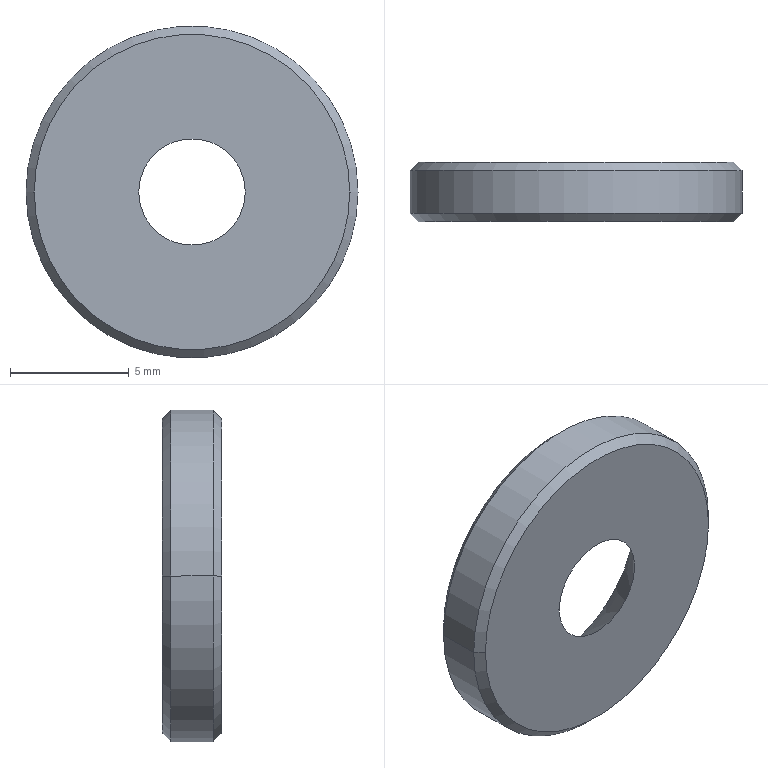Part | NX | 1 solid | 10 faces | box 14 x 2.5 x 14 mm | volume 279.245 mm3 | cone 6 | cylinder 2 | plane 2 | commonest cylinder face diameters 14 x2
STEP:
#1=CARTESIAN_POINT('',(-4.75,2.5,0.));
#2=VERTEX_POINT('',#1);
#3=CARTESIAN_POINT('',(4.75,2.5,0.));
#4=VERTEX_POINT('',#3);
#5=CARTESIAN_POINT('',(0.,2.5,0.));
#6=DIRECTION('',(0.,1.,0.));
#7=DIRECTION('',(1.,0.,0.));
#8=AXIS2_PLACEMENT_3D('',#5,#6,#7);
#9=CIRCLE('',#8,4.75);
#10=EDGE_CURVE('',#2,#4,#9,.T.);
#11=ORIENTED_EDGE('',*,*,#10,.T.);
#12=CARTESIAN_POINT('',(2.25,0.,0.));
#13=VERTEX_POINT('',#12);
#14=CARTESIAN_POINT('',(3.5,1.25,0.));
#15=DIRECTION('',(0.7071,0.7071,0.));
#16=VECTOR('',#15,1000.);
#17=LINE('',#14,#16);
#18=EDGE_CURVE('',#13,#4,#17,.T.);
#19=ORIENTED_EDGE('',*,*,#18,.F.);
#20=CARTESIAN_POINT('',(-2.25,0.,0.));
#21=VERTEX_POINT('',#20);
#22=CARTESIAN_POINT('',(0.,0.,0.));
#23=DIRECTION('',(0.,1.,0.));
#24=DIRECTION('',(1.,0.,0.));
#25=AXIS2_PLACEMENT_3D('',#22,#23,#24);
#26=CIRCLE('',#25,2.25);
#27=EDGE_CURVE('',#21,#13,#26,.T.);
#28=ORIENTED_EDGE('',*,*,#27,.F.);
#29=CARTESIAN_POINT('',(-3.5,1.25,0.));
#30=DIRECTION('',(-0.7071,0.7071,0.));
#31=VECTOR('',#30,1000.);
#32=LINE('',#29,#31);
#33=EDGE_CURVE('',#21,#2,#32,.T.);
#34=ORIENTED_EDGE('',*,*,#33,.T.);
#35=EDGE_LOOP('',(#11,#19,#28,#34));
#36=FACE_BOUND('',#35,.T.);
#37=CARTESIAN_POINT('',(0.,1.25,0.));
#38=DIRECTION('',(0.,1.,0.));
#39=DIRECTION('',(1.,0.,0.));
#40=AXIS2_PLACEMENT_3D('',#37,#38,#39);
#41=CONICAL_SURFACE('',#40,3.5,0.7854);
#42=ADVANCED_FACE('',(#36),#41,.F.);
#43=CARTESIAN_POINT('',(7.,2.15,0.));
#44=VERTEX_POINT('',#43);
#45=CARTESIAN_POINT('',(-7.,2.15,0.));
#46=VERTEX_POINT('',#45);
#47=CARTESIAN_POINT('',(0.,2.15,0.));
#48=DIRECTION('',(0.,1.,0.));
#49=DIRECTION('',(1.,0.,0.));
#50=AXIS2_PLACEMENT_3D('',#47,#48,#49);
#51=CIRCLE('',#50,7.);
#52=EDGE_CURVE('',#44,#46,#51,.T.);
#53=ORIENTED_EDGE('',*,*,#52,.T.);
#54=CARTESIAN_POINT('',(-6.65,2.5,0.));
#55=VERTEX_POINT('',#54);
#56=CARTESIAN_POINT('',(-6.825,2.325,0.));
#57=DIRECTION('',(-0.7071,-0.7071,0.));
#58=VECTOR('',#57,1000.);
#59=LINE('',#56,#58);
#60=EDGE_CURVE('',#46,#55,#59,.F.);
#61=ORIENTED_EDGE('',*,*,#60,.T.);
#62=CARTESIAN_POINT('',(6.65,2.5,0.));
#63=VERTEX_POINT('',#62);
#64=CARTESIAN_POINT('',(0.,2.5,0.));
#65=DIRECTION('',(0.,1.,0.));
#66=DIRECTION('',(1.,0.,0.));
#67=AXIS2_PLACEMENT_3D('',#64,#65,#66);
#68=CIRCLE('',#67,6.65);
#69=EDGE_CURVE('',#63,#55,#68,.T.);
#70=ORIENTED_EDGE('',*,*,#69,.F.);
#71=CARTESIAN_POINT('',(6.825,2.325,0.));
#72=DIRECTION('',(0.7071,-0.7071,0.));
#73=VECTOR('',#72,1000.);
#74=LINE('',#71,#73);
#75=EDGE_CURVE('',#44,#63,#74,.F.);
#76=ORIENTED_EDGE('',*,*,#75,.F.);
#77=EDGE_LOOP('',(#53,#61,#70,#76));
#78=FACE_BOUND('',#77,.T.);
#79=CARTESIAN_POINT('',(0.,2.325,0.));
#80=DIRECTION('',(0.,-1.,0.));
#81=DIRECTION('',(-1.,0.,0.));
#82=AXIS2_PLACEMENT_3D('',#79,#80,#81);
#83=CONICAL_SURFACE('',#82,6.825,0.7854);
#84=ADVANCED_FACE('',(#78),#83,.T.);
#85=CARTESIAN_POINT('',(7.,0.35,0.));
#86=VERTEX_POINT('',#85);
#87=CARTESIAN_POINT('',(-7.,0.35,0.));
#88=VERTEX_POINT('',#87);
#89=CARTESIAN_POINT('',(0.,0.35,0.));
#90=DIRECTION('',(0.,1.,0.));
#91=DIRECTION('',(1.,0.,0.));
#92=AXIS2_PLACEMENT_3D('',#89,#90,#91);
#93=CIRCLE('',#92,7.);
#94=EDGE_CURVE('',#86,#88,#93,.T.);
#95=ORIENTED_EDGE('',*,*,#94,.T.);
#96=CARTESIAN_POINT('',(-7.,1.25,0.));
#97=DIRECTION('',(0.,-1.,0.));
#98=VECTOR('',#97,1000.);
#99=LINE('',#96,#98);
#100=EDGE_CURVE('',#46,#88,#99,.T.);
#101=ORIENTED_EDGE('',*,*,#100,.F.);
#102=ORIENTED_EDGE('',*,*,#52,.F.);
#103=CARTESIAN_POINT('',(7.,1.25,0.));
#104=DIRECTION('',(0.,-1.,0.));
#105=VECTOR('',#104,1000.);
#106=LINE('',#103,#105);
#107=EDGE_CURVE('',#44,#86,#106,.T.);
#108=ORIENTED_EDGE('',*,*,#107,.T.);
#109=EDGE_LOOP('',(#95,#101,#102,#108));
#110=FACE_BOUND('',#109,.T.);
#111=CARTESIAN_POINT('',(0.,1.25,0.));
#112=DIRECTION('',(0.,-1.,0.));
#113=DIRECTION('',(1.,0.,0.));
#114=AXIS2_PLACEMENT_3D('',#111,#112,#113);
#115=CYLINDRICAL_SURFACE('',#114,7.);
#116=ADVANCED_FACE('',(#110),#115,.T.);
#117=ORIENTED_EDGE('',*,*,#94,.F.);
#118=CARTESIAN_POINT('',(6.65,0.,0.));
#119=VERTEX_POINT('',#118);
#120=CARTESIAN_POINT('',(6.825,0.175,0.));
#121=DIRECTION('',(0.7071,0.7071,0.));
#122=VECTOR('',#121,1000.);
#123=LINE('',#120,#122);
#124=EDGE_CURVE('',#119,#86,#123,.T.);
#125=ORIENTED_EDGE('',*,*,#124,.F.);
#126=CARTESIAN_POINT('',(-6.65,0.,0.));
#127=VERTEX_POINT('',#126);
#128=CARTESIAN_POINT('',(0.,0.,0.));
#129=DIRECTION('',(0.,1.,0.));
#130=DIRECTION('',(1.,0.,0.));
#131=AXIS2_PLACEMENT_3D('',#128,#129,#130);
#132=CIRCLE('',#131,6.65);
#133=EDGE_CURVE('',#119,#127,#132,.T.);
#134=ORIENTED_EDGE('',*,*,#133,.T.);
#135=CARTESIAN_POINT('',(-6.825,0.175,0.));
#136=DIRECTION('',(-0.7071,0.7071,0.));
#137=VECTOR('',#136,1000.);
#138=LINE('',#135,#137);
#139=EDGE_CURVE('',#127,#88,#138,.T.);
#140=ORIENTED_EDGE('',*,*,#139,.T.);
#141=EDGE_LOOP('',(#117,#125,#134,#140));
#142=FACE_BOUND('',#141,.T.);
#143=CARTESIAN_POINT('',(0.,0.175,0.));
#144=DIRECTION('',(0.,1.,0.));
#145=DIRECTION('',(1.,0.,0.));
#146=AXIS2_PLACEMENT_3D('',#143,#144,#145);
#147=CONICAL_SURFACE('',#146,6.825,0.7854);
#148=ADVANCED_FACE('',(#142),#147,.T.);
#149=CARTESIAN_POINT('',(0.,2.5,0.));
#150=DIRECTION('',(0.,1.,0.));
#151=DIRECTION('',(1.,0.,0.));
#152=AXIS2_PLACEMENT_3D('',#149,#150,#151);
#153=CIRCLE('',#152,6.65);
#154=EDGE_CURVE('',#55,#63,#153,.T.);
#155=ORIENTED_EDGE('',*,*,#154,.T.);
#156=ORIENTED_EDGE('',*,*,#69,.T.);
#157=EDGE_LOOP('',(#155,#156));
#158=FACE_BOUND('',#157,.T.);
#159=ORIENTED_EDGE('',*,*,#10,.F.);
#160=CARTESIAN_POINT('',(0.,2.5,0.));
#161=DIRECTION('',(0.,1.,0.));
#162=DIRECTION('',(1.,0.,0.));
#163=AXIS2_PLACEMENT_3D('',#160,#161,#162);
#164=CIRCLE('',#163,4.75);
#165=EDGE_CURVE('',#4,#2,#164,.T.);
#166=ORIENTED_EDGE('',*,*,#165,.F.);
#167=EDGE_LOOP('',(#159,#166));
#168=FACE_BOUND('',#167,.T.);
#169=CARTESIAN_POINT('',(5.7,2.5,0.));
#170=DIRECTION('',(0.,1.,0.));
#171=DIRECTION('',(1.,0.,0.));
#172=AXIS2_PLACEMENT_3D('',#169,#170,#171);
#173=PLANE('',#172);
#174=ADVANCED_FACE('',(#158,#168),#173,.T.);
#175=CARTESIAN_POINT('',(0.,0.,0.));
#176=DIRECTION('',(0.,1.,0.));
#177=DIRECTION('',(1.,0.,0.));
#178=AXIS2_PLACEMENT_3D('',#175,#176,#177);
#179=CIRCLE('',#178,6.65);
#180=EDGE_CURVE('',#127,#119,#179,.T.);
#181=ORIENTED_EDGE('',*,*,#180,.F.);
#182=ORIENTED_EDGE('',*,*,#133,.F.);
#183=EDGE_LOOP('',(#181,#182));
#184=FACE_BOUND('',#183,.T.);
#185=CARTESIAN_POINT('',(0.,0.,0.));
#186=DIRECTION('',(0.,1.,0.));
#187=DIRECTION('',(1.,0.,0.));
#188=AXIS2_PLACEMENT_3D('',#185,#186,#187);
#189=CIRCLE('',#188,2.25);
#190=EDGE_CURVE('',#13,#21,#189,.T.);
#191=ORIENTED_EDGE('',*,*,#190,.T.);
#192=ORIENTED_EDGE('',*,*,#27,.T.);
#193=EDGE_LOOP('',(#191,#192));
#194=FACE_BOUND('',#193,.T.);
#195=CARTESIAN_POINT('',(4.45,0.,0.));
#196=DIRECTION('',(0.,-1.,0.));
#197=DIRECTION('',(-1.,0.,0.));
#198=AXIS2_PLACEMENT_3D('',#195,#196,#197);
#199=PLANE('',#198);
#200=ADVANCED_FACE('',(#184,#194),#199,.T.);
#201=ORIENTED_EDGE('',*,*,#180,.T.);
#202=ORIENTED_EDGE('',*,*,#124,.T.);
#203=CARTESIAN_POINT('',(0.,0.35,0.));
#204=DIRECTION('',(0.,1.,0.));
#205=DIRECTION('',(1.,0.,0.));
#206=AXIS2_PLACEMENT_3D('',#203,#204,#205);
#207=CIRCLE('',#206,7.);
#208=EDGE_CURVE('',#88,#86,#207,.T.);
#209=ORIENTED_EDGE('',*,*,#208,.F.);
#210=ORIENTED_EDGE('',*,*,#139,.F.);
#211=EDGE_LOOP('',(#201,#202,#209,#210));
#212=FACE_BOUND('',#211,.T.);
#213=CARTESIAN_POINT('',(0.,0.175,0.));
#214=DIRECTION('',(0.,1.,0.));
#215=DIRECTION('',(1.,0.,0.));
#216=AXIS2_PLACEMENT_3D('',#213,#214,#215);
#217=CONICAL_SURFACE('',#216,6.825,0.7854);
#218=ADVANCED_FACE('',(#212),#217,.T.);
#219=ORIENTED_EDGE('',*,*,#107,.F.);
#220=CARTESIAN_POINT('',(0.,2.15,0.));
#221=DIRECTION('',(0.,1.,0.));
#222=DIRECTION('',(1.,0.,0.));
#223=AXIS2_PLACEMENT_3D('',#220,#221,#222);
#224=CIRCLE('',#223,7.);
#225=EDGE_CURVE('',#46,#44,#224,.T.);
#226=ORIENTED_EDGE('',*,*,#225,.F.);
#227=ORIENTED_EDGE('',*,*,#100,.T.);
#228=ORIENTED_EDGE('',*,*,#208,.T.);
#229=EDGE_LOOP('',(#219,#226,#227,#228));
#230=FACE_BOUND('',#229,.T.);
#231=CARTESIAN_POINT('',(0.,1.25,0.));
#232=DIRECTION('',(0.,-1.,0.));
#233=DIRECTION('',(1.,0.,0.));
#234=AXIS2_PLACEMENT_3D('',#231,#232,#233);
#235=CYLINDRICAL_SURFACE('',#234,7.);
#236=ADVANCED_FACE('',(#230),#235,.T.);
#237=ORIENTED_EDGE('',*,*,#154,.F.);
#238=ORIENTED_EDGE('',*,*,#60,.F.);
#239=ORIENTED_EDGE('',*,*,#225,.T.);
#240=ORIENTED_EDGE('',*,*,#75,.T.);
#241=EDGE_LOOP('',(#237,#238,#239,#240));
#242=FACE_BOUND('',#241,.T.);
#243=CARTESIAN_POINT('',(0.,2.325,0.));
#244=DIRECTION('',(0.,-1.,0.));
#245=DIRECTION('',(-1.,0.,0.));
#246=AXIS2_PLACEMENT_3D('',#243,#244,#245);
#247=CONICAL_SURFACE('',#246,6.825,0.7854);
#248=ADVANCED_FACE('',(#242),#247,.T.);
#249=ORIENTED_EDGE('',*,*,#190,.F.);
#250=ORIENTED_EDGE('',*,*,#18,.T.);
#251=ORIENTED_EDGE('',*,*,#165,.T.);
#252=ORIENTED_EDGE('',*,*,#33,.F.);
#253=EDGE_LOOP('',(#249,#250,#251,#252));
#254=FACE_BOUND('',#253,.T.);
#255=CARTESIAN_POINT('',(0.,1.25,0.));
#256=DIRECTION('',(0.,1.,0.));
#257=DIRECTION('',(1.,0.,0.));
#258=AXIS2_PLACEMENT_3D('',#255,#256,#257);
#259=CONICAL_SURFACE('',#258,3.5,0.7854);
#260=ADVANCED_FACE('',(#254),#259,.F.);
#261=CLOSED_SHELL('',(#42,#84,#116,#148,#174,#200,#218,#236,#248,#260));
#262=MANIFOLD_SOLID_BREP('',#261);
#263=(LENGTH_UNIT()NAMED_UNIT(*)SI_UNIT(.MILLI.,.METRE.));
#264=UNCERTAINTY_MEASURE_WITH_UNIT(LENGTH_MEASURE(0.00001),#263,'','');
#265=(NAMED_UNIT(*)PLANE_ANGLE_UNIT()SI_UNIT($,.RADIAN.));
#266=(NAMED_UNIT(*)SI_UNIT($,.STERADIAN.)SOLID_ANGLE_UNIT());
#267=(GEOMETRIC_REPRESENTATION_CONTEXT(3)GLOBAL_UNCERTAINTY_ASSIGNED_CONTEXT((#264))GLOBAL_UNIT_ASSIGNED_CONTEXT((#263,#265,#266))REPRESENTATION_CONTEXT('',''));
#268=ADVANCED_BREP_SHAPE_REPRESENTATION('',(#262),#267);